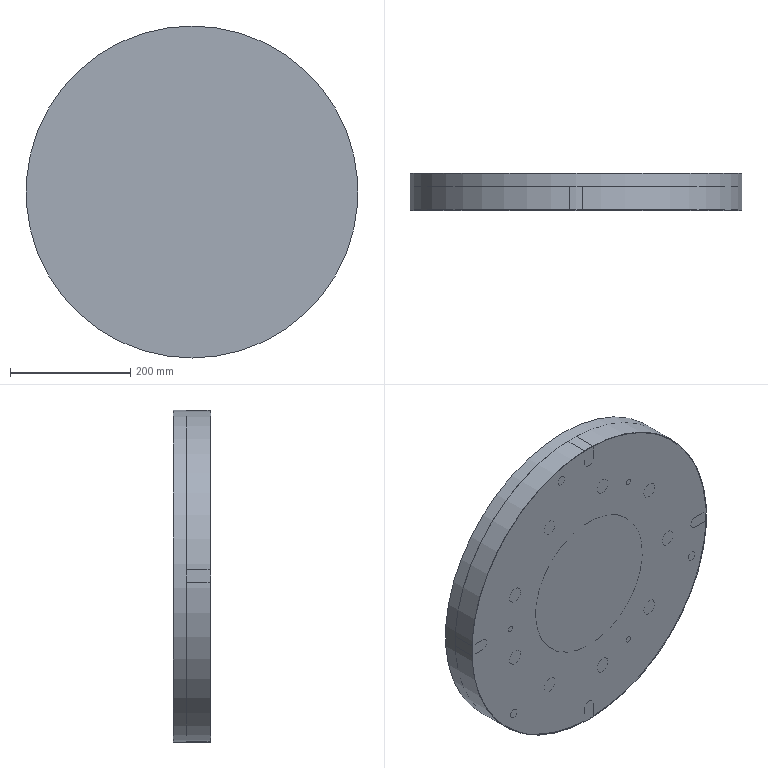NC program | NX | posted with a generic post | part box 552 x 62 x 552 mm
Whole program:
N10 G17 G21 G94 G90
(CAVITY_MILL_COPY , TOOL : D18)
N12 T02 M6
N14 G54
N16 G17 G0 G90 X1.013 Y-305.278 S900 M3
N18 G43 Z19. H2
N20 Z-60.
N22 G94 G1 Z-63. F60.
N24 G41 X1. Y-274.822 D2
N26 Y-250.
N28 G3 X0. Y-249. R1.
N30 X-1. Y-250. R1.
N32 G1 Y-274.822
N34 X-1.011 Y-300.278
N36 G40
N38 X-1.013 Y-305.278
N40 Z-60.
N42 G0 Z19.
N44 M5
N46 M2